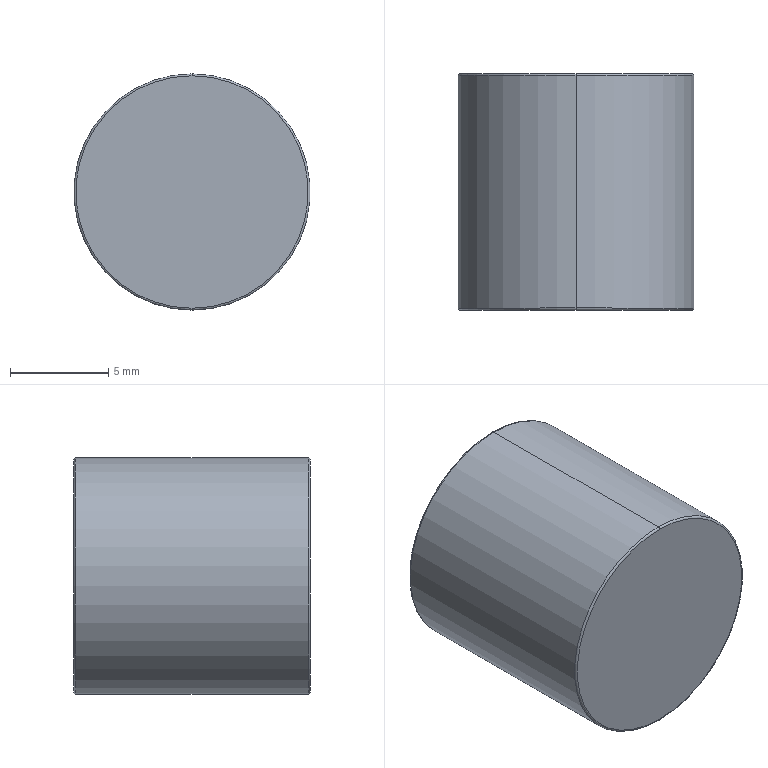Part | SolidWorks | features Fillet 1, RefAxis 1, Revolution 1 | 1 solid | 8 faces | box 12 x 12 x 12 mm | volume 1357 mm3 | torus 4 | cylinder 2 | plane 2 | commonest cylinder face diameters 12 x2
STEP:
#1=CARTESIAN_POINT('',(0.,6.,5.9));
#2=VERTEX_POINT('',#1);
#3=CARTESIAN_POINT('',(0.,6.,-5.9));
#4=VERTEX_POINT('',#3);
#5=CARTESIAN_POINT('',(0.,6.,0.));
#6=DIRECTION('',(0.,1.,0.));
#7=DIRECTION('',(0.,0.,-1.));
#8=AXIS2_PLACEMENT_3D('',#5,#6,#7);
#9=CIRCLE('',#8,5.9);
#10=EDGE_CURVE('',#2,#4,#9,.T.);
#11=ORIENTED_EDGE('',*,*,#10,.F.);
#12=CARTESIAN_POINT('',(0.,5.9,6.));
#13=VERTEX_POINT('',#12);
#14=CARTESIAN_POINT('',(0.,5.9,5.9));
#15=DIRECTION('',(1.,0.,0.));
#16=DIRECTION('',(0.,0.,-1.));
#17=AXIS2_PLACEMENT_3D('',#14,#15,#16);
#18=CIRCLE('',#17,0.1);
#19=EDGE_CURVE('',#2,#13,#18,.T.);
#20=ORIENTED_EDGE('',*,*,#19,.T.);
#21=CARTESIAN_POINT('',(0.,5.9,-6.));
#22=VERTEX_POINT('',#21);
#23=CARTESIAN_POINT('',(0.,5.9,0.));
#24=DIRECTION('',(0.,-1.,0.));
#25=DIRECTION('',(0.,0.,-1.));
#26=AXIS2_PLACEMENT_3D('',#23,#24,#25);
#27=CIRCLE('',#26,6.);
#28=EDGE_CURVE('',#22,#13,#27,.T.);
#29=ORIENTED_EDGE('',*,*,#28,.F.);
#30=CARTESIAN_POINT('',(0.,5.9,-5.9));
#31=DIRECTION('',(-1.,0.,0.));
#32=DIRECTION('',(0.,0.,1.));
#33=AXIS2_PLACEMENT_3D('',#30,#31,#32);
#34=CIRCLE('',#33,0.1);
#35=EDGE_CURVE('',#4,#22,#34,.T.);
#36=ORIENTED_EDGE('',*,*,#35,.F.);
#37=EDGE_LOOP('',(#11,#20,#29,#36));
#38=FACE_OUTER_BOUND('',#37,.T.);
#39=CARTESIAN_POINT('',(0.,5.9,0.));
#40=DIRECTION('',(0.,-1.,0.));
#41=DIRECTION('',(0.,0.,-1.));
#42=AXIS2_PLACEMENT_3D('',#39,#40,#41);
#43=TOROIDAL_SURFACE('',#42,5.9,0.1);
#44=ADVANCED_FACE('',(#38),#43,.T.);
#45=CARTESIAN_POINT('',(0.,-6.,-5.9));
#46=VERTEX_POINT('',#45);
#47=CARTESIAN_POINT('',(0.,-6.,5.9));
#48=VERTEX_POINT('',#47);
#49=CARTESIAN_POINT('',(0.,-6.,0.));
#50=DIRECTION('',(0.,-1.,0.));
#51=DIRECTION('',(0.,0.,1.));
#52=AXIS2_PLACEMENT_3D('',#49,#50,#51);
#53=CIRCLE('',#52,5.9);
#54=EDGE_CURVE('',#46,#48,#53,.T.);
#55=ORIENTED_EDGE('',*,*,#54,.F.);
#56=CARTESIAN_POINT('',(0.,-5.9,-6.));
#57=VERTEX_POINT('',#56);
#58=CARTESIAN_POINT('',(0.,-5.9,-5.9));
#59=DIRECTION('',(1.,0.,0.));
#60=DIRECTION('',(0.,0.,-1.));
#61=AXIS2_PLACEMENT_3D('',#58,#59,#60);
#62=CIRCLE('',#61,0.1);
#63=EDGE_CURVE('',#46,#57,#62,.T.);
#64=ORIENTED_EDGE('',*,*,#63,.T.);
#65=CARTESIAN_POINT('',(0.,-5.9,6.));
#66=VERTEX_POINT('',#65);
#67=CARTESIAN_POINT('',(0.,-5.9,0.));
#68=DIRECTION('',(0.,1.,0.));
#69=DIRECTION('',(0.,0.,1.));
#70=AXIS2_PLACEMENT_3D('',#67,#68,#69);
#71=CIRCLE('',#70,6.);
#72=EDGE_CURVE('',#66,#57,#71,.T.);
#73=ORIENTED_EDGE('',*,*,#72,.F.);
#74=CARTESIAN_POINT('',(0.,-5.9,5.9));
#75=DIRECTION('',(-1.,0.,0.));
#76=DIRECTION('',(0.,0.,1.));
#77=AXIS2_PLACEMENT_3D('',#74,#75,#76);
#78=CIRCLE('',#77,0.1);
#79=EDGE_CURVE('',#48,#66,#78,.T.);
#80=ORIENTED_EDGE('',*,*,#79,.F.);
#81=EDGE_LOOP('',(#55,#64,#73,#80));
#82=FACE_OUTER_BOUND('',#81,.T.);
#83=CARTESIAN_POINT('',(0.,-5.9,0.));
#84=DIRECTION('',(0.,1.,0.));
#85=DIRECTION('',(0.,0.,1.));
#86=AXIS2_PLACEMENT_3D('',#83,#84,#85);
#87=TOROIDAL_SURFACE('',#86,5.9,0.1);
#88=ADVANCED_FACE('',(#82),#87,.T.);
#89=ORIENTED_EDGE('',*,*,#72,.T.);
#90=CARTESIAN_POINT('',(0.,6.,-6.));
#91=DIRECTION('',(0.,1.,0.));
#92=VECTOR('',#91,1000.);
#93=LINE('',#90,#92);
#94=EDGE_CURVE('',#57,#22,#93,.T.);
#95=ORIENTED_EDGE('',*,*,#94,.T.);
#96=ORIENTED_EDGE('',*,*,#28,.T.);
#97=CARTESIAN_POINT('',(0.,6.,6.));
#98=DIRECTION('',(0.,1.,0.));
#99=VECTOR('',#98,1000.);
#100=LINE('',#97,#99);
#101=EDGE_CURVE('',#66,#13,#100,.T.);
#102=ORIENTED_EDGE('',*,*,#101,.F.);
#103=EDGE_LOOP('',(#89,#95,#96,#102));
#104=FACE_OUTER_BOUND('',#103,.T.);
#105=CARTESIAN_POINT('',(0.,6.,0.));
#106=DIRECTION('',(0.,1.,0.));
#107=DIRECTION('',(0.,0.,1.));
#108=AXIS2_PLACEMENT_3D('',#105,#106,#107);
#109=CYLINDRICAL_SURFACE('',#108,6.);
#110=ADVANCED_FACE('',(#104),#109,.T.);
#111=ORIENTED_EDGE('',*,*,#94,.F.);
#112=CARTESIAN_POINT('',(0.,-5.9,0.));
#113=DIRECTION('',(0.,1.,0.));
#114=DIRECTION('',(0.,0.,1.));
#115=AXIS2_PLACEMENT_3D('',#112,#113,#114);
#116=CIRCLE('',#115,6.);
#117=EDGE_CURVE('',#57,#66,#116,.T.);
#118=ORIENTED_EDGE('',*,*,#117,.T.);
#119=ORIENTED_EDGE('',*,*,#101,.T.);
#120=CARTESIAN_POINT('',(0.,5.9,0.));
#121=DIRECTION('',(0.,-1.,0.));
#122=DIRECTION('',(0.,0.,-1.));
#123=AXIS2_PLACEMENT_3D('',#120,#121,#122);
#124=CIRCLE('',#123,6.);
#125=EDGE_CURVE('',#13,#22,#124,.T.);
#126=ORIENTED_EDGE('',*,*,#125,.T.);
#127=EDGE_LOOP('',(#111,#118,#119,#126));
#128=FACE_OUTER_BOUND('',#127,.T.);
#129=CARTESIAN_POINT('',(0.,6.,0.));
#130=DIRECTION('',(0.,1.,0.));
#131=DIRECTION('',(0.,0.,1.));
#132=AXIS2_PLACEMENT_3D('',#129,#130,#131);
#133=CYLINDRICAL_SURFACE('',#132,6.);
#134=ADVANCED_FACE('',(#128),#133,.T.);
#135=CARTESIAN_POINT('',(0.,6.,0.));
#136=DIRECTION('',(0.,1.,0.));
#137=DIRECTION('',(0.,0.,-1.));
#138=AXIS2_PLACEMENT_3D('',#135,#136,#137);
#139=CIRCLE('',#138,5.9);
#140=EDGE_CURVE('',#4,#2,#139,.T.);
#141=ORIENTED_EDGE('',*,*,#140,.T.);
#142=ORIENTED_EDGE('',*,*,#10,.T.);
#143=EDGE_LOOP('',(#141,#142));
#144=FACE_OUTER_BOUND('',#143,.T.);
#145=CARTESIAN_POINT('',(0.,6.,0.));
#146=DIRECTION('',(0.,-1.,0.));
#147=DIRECTION('',(0.,0.,-1.));
#148=AXIS2_PLACEMENT_3D('',#145,#146,#147);
#149=PLANE('',#148);
#150=ADVANCED_FACE('',(#144),#149,.F.);
#151=CARTESIAN_POINT('',(0.,-6.,0.));
#152=DIRECTION('',(0.,-1.,0.));
#153=DIRECTION('',(0.,0.,1.));
#154=AXIS2_PLACEMENT_3D('',#151,#152,#153);
#155=CIRCLE('',#154,5.9);
#156=EDGE_CURVE('',#48,#46,#155,.T.);
#157=ORIENTED_EDGE('',*,*,#156,.T.);
#158=ORIENTED_EDGE('',*,*,#54,.T.);
#159=EDGE_LOOP('',(#157,#158));
#160=FACE_OUTER_BOUND('',#159,.T.);
#161=CARTESIAN_POINT('',(0.,-6.,0.));
#162=DIRECTION('',(0.,1.,0.));
#163=DIRECTION('',(0.,0.,1.));
#164=AXIS2_PLACEMENT_3D('',#161,#162,#163);
#165=PLANE('',#164);
#166=ADVANCED_FACE('',(#160),#165,.F.);
#167=ORIENTED_EDGE('',*,*,#63,.F.);
#168=ORIENTED_EDGE('',*,*,#156,.F.);
#169=ORIENTED_EDGE('',*,*,#79,.T.);
#170=ORIENTED_EDGE('',*,*,#117,.F.);
#171=EDGE_LOOP('',(#167,#168,#169,#170));
#172=FACE_OUTER_BOUND('',#171,.T.);
#173=CARTESIAN_POINT('',(0.,-5.9,0.));
#174=DIRECTION('',(0.,1.,0.));
#175=DIRECTION('',(0.,0.,1.));
#176=AXIS2_PLACEMENT_3D('',#173,#174,#175);
#177=TOROIDAL_SURFACE('',#176,5.9,0.1);
#178=ADVANCED_FACE('',(#172),#177,.T.);
#179=ORIENTED_EDGE('',*,*,#19,.F.);
#180=ORIENTED_EDGE('',*,*,#140,.F.);
#181=ORIENTED_EDGE('',*,*,#35,.T.);
#182=ORIENTED_EDGE('',*,*,#125,.F.);
#183=EDGE_LOOP('',(#179,#180,#181,#182));
#184=FACE_OUTER_BOUND('',#183,.T.);
#185=CARTESIAN_POINT('',(0.,5.9,0.));
#186=DIRECTION('',(0.,-1.,0.));
#187=DIRECTION('',(0.,0.,-1.));
#188=AXIS2_PLACEMENT_3D('',#185,#186,#187);
#189=TOROIDAL_SURFACE('',#188,5.9,0.1);
#190=ADVANCED_FACE('',(#184),#189,.T.);
#191=CLOSED_SHELL('',(#44,#88,#110,#134,#150,#166,#178,#190));
#192=MANIFOLD_SOLID_BREP('',#191);
#193=CARTESIAN_POINT('',(0.,0.,0.));
#194=DIRECTION('',(0.,0.,1.));
#195=DIRECTION('',(1.,0.,0.));
#196=AXIS2_PLACEMENT_3D('',#193,#194,#195);
#197=(LENGTH_UNIT()NAMED_UNIT(*)SI_UNIT(.MILLI.,.METRE.));
#198=UNCERTAINTY_MEASURE_WITH_UNIT(LENGTH_MEASURE(0.00001),#197,'','');
#199=(NAMED_UNIT(*)PLANE_ANGLE_UNIT()SI_UNIT($,.RADIAN.));
#200=(NAMED_UNIT(*)SI_UNIT($,.STERADIAN.)SOLID_ANGLE_UNIT());
#201=(GEOMETRIC_REPRESENTATION_CONTEXT(3)GLOBAL_UNCERTAINTY_ASSIGNED_CONTEXT((#198))GLOBAL_UNIT_ASSIGNED_CONTEXT((#197,#199,#200))REPRESENTATION_CONTEXT('',''));
#202=ADVANCED_BREP_SHAPE_REPRESENTATION('',(#192,#196),#201);